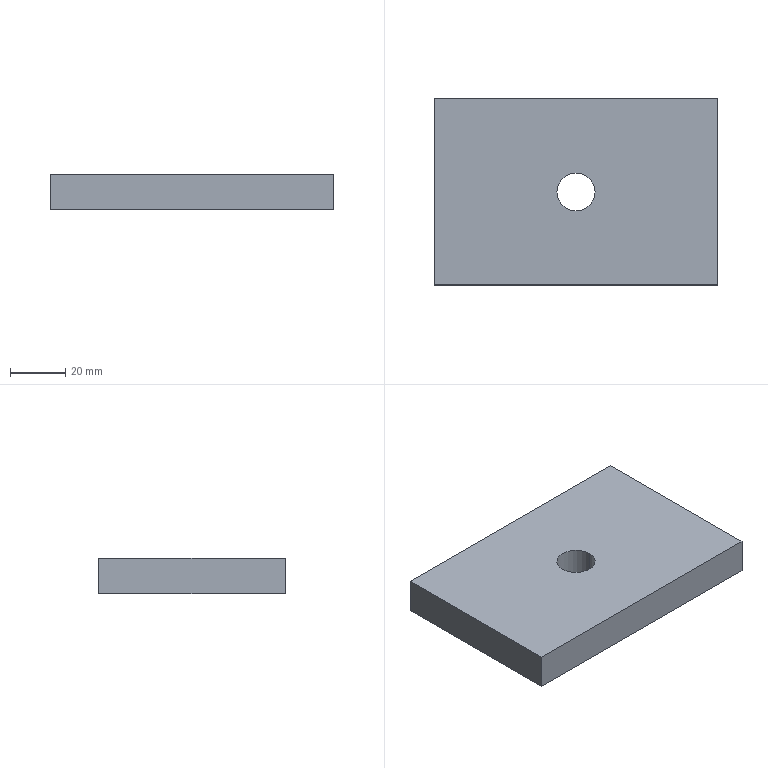Part | SolidWorks | features BaseBody 1 | 1 solid | 8 faces | box 103 x 67.6 x 13 mm | volume 88562 mm3 | plane 6 | cylinder 2 | commonest cylinder face diameters 13.835 x2
STEP:
#1=CARTESIAN_POINT('',(34.779,28.356,0.));
#2=VERTEX_POINT('',#1);
#3=CARTESIAN_POINT('',(20.944,28.356,0.));
#4=VERTEX_POINT('',#3);
#5=CARTESIAN_POINT('',(27.861,28.356,0.));
#6=DIRECTION('',(0.,0.,-1.));
#7=DIRECTION('',(1.,0.,0.));
#8=AXIS2_PLACEMENT_3D('',#5,#6,#7);
#9=CIRCLE('',#8,6.918);
#10=EDGE_CURVE('',#2,#4,#9,.T.);
#11=ORIENTED_EDGE('',*,*,#10,.T.);
#12=CARTESIAN_POINT('',(20.944,28.356,13.));
#13=VERTEX_POINT('',#12);
#14=CARTESIAN_POINT('',(20.944,28.356,-110.886));
#15=DIRECTION('',(0.,0.,1.));
#16=VECTOR('',#15,1000.);
#17=LINE('',#14,#16);
#18=EDGE_CURVE('',#4,#13,#17,.T.);
#19=ORIENTED_EDGE('',*,*,#18,.T.);
#20=CARTESIAN_POINT('',(34.779,28.356,13.));
#21=VERTEX_POINT('',#20);
#22=CARTESIAN_POINT('',(27.861,28.356,13.));
#23=DIRECTION('',(0.,0.,-1.));
#24=DIRECTION('',(1.,0.,0.));
#25=AXIS2_PLACEMENT_3D('',#22,#23,#24);
#26=CIRCLE('',#25,6.918);
#27=EDGE_CURVE('',#21,#13,#26,.T.);
#28=ORIENTED_EDGE('',*,*,#27,.F.);
#29=CARTESIAN_POINT('',(34.779,28.356,-110.886));
#30=DIRECTION('',(0.,0.,1.));
#31=VECTOR('',#30,1000.);
#32=LINE('',#29,#31);
#33=EDGE_CURVE('',#2,#21,#32,.T.);
#34=ORIENTED_EDGE('',*,*,#33,.F.);
#35=EDGE_LOOP('',(#11,#19,#28,#34));
#36=FACE_OUTER_BOUND('',#35,.T.);
#37=CARTESIAN_POINT('',(27.861,28.356,-110.886));
#38=DIRECTION('',(0.,0.,1.));
#39=DIRECTION('',(1.,0.,0.));
#40=AXIS2_PLACEMENT_3D('',#37,#38,#39);
#41=CYLINDRICAL_SURFACE('',#40,6.918);
#42=ADVANCED_FACE('',(#36),#41,.F.);
#43=ORIENTED_EDGE('',*,*,#10,.F.);
#44=CARTESIAN_POINT('',(27.861,28.356,0.));
#45=DIRECTION('',(0.,0.,-1.));
#46=DIRECTION('',(1.,0.,0.));
#47=AXIS2_PLACEMENT_3D('',#44,#45,#46);
#48=CIRCLE('',#47,6.918);
#49=EDGE_CURVE('',#4,#2,#48,.T.);
#50=ORIENTED_EDGE('',*,*,#49,.F.);
#51=EDGE_LOOP('',(#43,#50));
#52=FACE_BOUND('',#51,.T.);
#53=CARTESIAN_POINT('',(79.361,-5.444,0.));
#54=VERTEX_POINT('',#53);
#55=CARTESIAN_POINT('',(79.361,62.156,0.));
#56=VERTEX_POINT('',#55);
#57=CARTESIAN_POINT('',(79.361,28.356,0.));
#58=DIRECTION('',(0.,1.,0.));
#59=VECTOR('',#58,1000.);
#60=LINE('',#57,#59);
#61=EDGE_CURVE('',#54,#56,#60,.T.);
#62=ORIENTED_EDGE('',*,*,#61,.F.);
#63=CARTESIAN_POINT('',(-23.639,-5.444,0.));
#64=VERTEX_POINT('',#63);
#65=CARTESIAN_POINT('',(27.861,-5.444,0.));
#66=DIRECTION('',(1.,0.,0.));
#67=VECTOR('',#66,1000.);
#68=LINE('',#65,#67);
#69=EDGE_CURVE('',#64,#54,#68,.T.);
#70=ORIENTED_EDGE('',*,*,#69,.F.);
#71=CARTESIAN_POINT('',(-23.639,62.156,0.));
#72=VERTEX_POINT('',#71);
#73=CARTESIAN_POINT('',(-23.639,28.356,0.));
#74=DIRECTION('',(0.,-1.,0.));
#75=VECTOR('',#74,1000.);
#76=LINE('',#73,#75);
#77=EDGE_CURVE('',#72,#64,#76,.T.);
#78=ORIENTED_EDGE('',*,*,#77,.F.);
#79=CARTESIAN_POINT('',(27.861,62.156,0.));
#80=DIRECTION('',(-1.,0.,0.));
#81=VECTOR('',#80,1000.);
#82=LINE('',#79,#81);
#83=EDGE_CURVE('',#56,#72,#82,.T.);
#84=ORIENTED_EDGE('',*,*,#83,.F.);
#85=EDGE_LOOP('',(#62,#70,#78,#84));
#86=FACE_OUTER_BOUND('',#85,.T.);
#87=CARTESIAN_POINT('',(27.861,28.356,0.));
#88=DIRECTION('',(0.,0.,1.));
#89=DIRECTION('',(1.,0.,0.));
#90=AXIS2_PLACEMENT_3D('',#87,#88,#89);
#91=PLANE('',#90);
#92=ADVANCED_FACE('',(#52,#86),#91,.F.);
#93=ORIENTED_EDGE('',*,*,#18,.F.);
#94=ORIENTED_EDGE('',*,*,#49,.T.);
#95=ORIENTED_EDGE('',*,*,#33,.T.);
#96=CARTESIAN_POINT('',(27.861,28.356,13.));
#97=DIRECTION('',(0.,0.,-1.));
#98=DIRECTION('',(1.,0.,0.));
#99=AXIS2_PLACEMENT_3D('',#96,#97,#98);
#100=CIRCLE('',#99,6.918);
#101=EDGE_CURVE('',#13,#21,#100,.T.);
#102=ORIENTED_EDGE('',*,*,#101,.F.);
#103=EDGE_LOOP('',(#93,#94,#95,#102));
#104=FACE_OUTER_BOUND('',#103,.T.);
#105=CARTESIAN_POINT('',(27.861,28.356,-110.886));
#106=DIRECTION('',(0.,0.,1.));
#107=DIRECTION('',(1.,0.,0.));
#108=AXIS2_PLACEMENT_3D('',#105,#106,#107);
#109=CYLINDRICAL_SURFACE('',#108,6.918);
#110=ADVANCED_FACE('',(#104),#109,.F.);
#111=ORIENTED_EDGE('',*,*,#83,.T.);
#112=CARTESIAN_POINT('',(-23.639,62.156,13.));
#113=VERTEX_POINT('',#112);
#114=CARTESIAN_POINT('',(-23.639,62.156,0.));
#115=DIRECTION('',(0.,0.,1.));
#116=VECTOR('',#115,1000.);
#117=LINE('',#114,#116);
#118=EDGE_CURVE('',#72,#113,#117,.T.);
#119=ORIENTED_EDGE('',*,*,#118,.T.);
#120=CARTESIAN_POINT('',(79.361,62.156,13.));
#121=VERTEX_POINT('',#120);
#122=CARTESIAN_POINT('',(-23.639,62.156,13.));
#123=DIRECTION('',(1.,0.,0.));
#124=VECTOR('',#123,1000.);
#125=LINE('',#122,#124);
#126=EDGE_CURVE('',#113,#121,#125,.T.);
#127=ORIENTED_EDGE('',*,*,#126,.T.);
#128=CARTESIAN_POINT('',(79.361,62.156,0.));
#129=DIRECTION('',(0.,0.,-1.));
#130=VECTOR('',#129,1000.);
#131=LINE('',#128,#130);
#132=EDGE_CURVE('',#121,#56,#131,.T.);
#133=ORIENTED_EDGE('',*,*,#132,.T.);
#134=EDGE_LOOP('',(#111,#119,#127,#133));
#135=FACE_OUTER_BOUND('',#134,.T.);
#136=CARTESIAN_POINT('',(-23.639,62.156,0.));
#137=DIRECTION('',(0.,1.,0.));
#138=DIRECTION('',(0.,0.,1.));
#139=AXIS2_PLACEMENT_3D('',#136,#137,#138);
#140=PLANE('',#139);
#141=ADVANCED_FACE('',(#135),#140,.T.);
#142=ORIENTED_EDGE('',*,*,#61,.T.);
#143=ORIENTED_EDGE('',*,*,#132,.F.);
#144=CARTESIAN_POINT('',(79.361,-5.444,13.));
#145=VERTEX_POINT('',#144);
#146=CARTESIAN_POINT('',(79.361,62.156,13.));
#147=DIRECTION('',(0.,-1.,0.));
#148=VECTOR('',#147,1000.);
#149=LINE('',#146,#148);
#150=EDGE_CURVE('',#121,#145,#149,.T.);
#151=ORIENTED_EDGE('',*,*,#150,.T.);
#152=CARTESIAN_POINT('',(79.361,-5.444,0.));
#153=DIRECTION('',(0.,0.,-1.));
#154=VECTOR('',#153,1000.);
#155=LINE('',#152,#154);
#156=EDGE_CURVE('',#145,#54,#155,.T.);
#157=ORIENTED_EDGE('',*,*,#156,.T.);
#158=EDGE_LOOP('',(#142,#143,#151,#157));
#159=FACE_OUTER_BOUND('',#158,.T.);
#160=CARTESIAN_POINT('',(79.361,62.156,0.));
#161=DIRECTION('',(1.,0.,0.));
#162=DIRECTION('',(0.,0.,-1.));
#163=AXIS2_PLACEMENT_3D('',#160,#161,#162);
#164=PLANE('',#163);
#165=ADVANCED_FACE('',(#159),#164,.T.);
#166=ORIENTED_EDGE('',*,*,#69,.T.);
#167=ORIENTED_EDGE('',*,*,#156,.F.);
#168=CARTESIAN_POINT('',(-23.639,-5.444,13.));
#169=VERTEX_POINT('',#168);
#170=CARTESIAN_POINT('',(79.361,-5.444,13.));
#171=DIRECTION('',(-1.,0.,0.));
#172=VECTOR('',#171,1000.);
#173=LINE('',#170,#172);
#174=EDGE_CURVE('',#145,#169,#173,.T.);
#175=ORIENTED_EDGE('',*,*,#174,.T.);
#176=CARTESIAN_POINT('',(-23.639,-5.444,0.));
#177=DIRECTION('',(0.,0.,-1.));
#178=VECTOR('',#177,1000.);
#179=LINE('',#176,#178);
#180=EDGE_CURVE('',#169,#64,#179,.T.);
#181=ORIENTED_EDGE('',*,*,#180,.T.);
#182=EDGE_LOOP('',(#166,#167,#175,#181));
#183=FACE_OUTER_BOUND('',#182,.T.);
#184=CARTESIAN_POINT('',(79.361,-5.444,0.));
#185=DIRECTION('',(0.,-1.,0.));
#186=DIRECTION('',(1.,0.,0.));
#187=AXIS2_PLACEMENT_3D('',#184,#185,#186);
#188=PLANE('',#187);
#189=ADVANCED_FACE('',(#183),#188,.T.);
#190=ORIENTED_EDGE('',*,*,#77,.T.);
#191=ORIENTED_EDGE('',*,*,#180,.F.);
#192=CARTESIAN_POINT('',(-23.639,-5.444,13.));
#193=DIRECTION('',(0.,1.,0.));
#194=VECTOR('',#193,1000.);
#195=LINE('',#192,#194);
#196=EDGE_CURVE('',#169,#113,#195,.T.);
#197=ORIENTED_EDGE('',*,*,#196,.T.);
#198=ORIENTED_EDGE('',*,*,#118,.F.);
#199=EDGE_LOOP('',(#190,#191,#197,#198));
#200=FACE_OUTER_BOUND('',#199,.T.);
#201=CARTESIAN_POINT('',(-23.639,-5.444,0.));
#202=DIRECTION('',(-1.,0.,0.));
#203=DIRECTION('',(0.,-1.,0.));
#204=AXIS2_PLACEMENT_3D('',#201,#202,#203);
#205=PLANE('',#204);
#206=ADVANCED_FACE('',(#200),#205,.T.);
#207=ORIENTED_EDGE('',*,*,#27,.T.);
#208=ORIENTED_EDGE('',*,*,#101,.T.);
#209=EDGE_LOOP('',(#207,#208));
#210=FACE_BOUND('',#209,.T.);
#211=ORIENTED_EDGE('',*,*,#196,.F.);
#212=ORIENTED_EDGE('',*,*,#174,.F.);
#213=ORIENTED_EDGE('',*,*,#150,.F.);
#214=ORIENTED_EDGE('',*,*,#126,.F.);
#215=EDGE_LOOP('',(#211,#212,#213,#214));
#216=FACE_OUTER_BOUND('',#215,.T.);
#217=CARTESIAN_POINT('',(27.861,28.356,13.));
#218=DIRECTION('',(0.,0.,1.));
#219=DIRECTION('',(1.,0.,0.));
#220=AXIS2_PLACEMENT_3D('',#217,#218,#219);
#221=PLANE('',#220);
#222=ADVANCED_FACE('',(#210,#216),#221,.T.);
#223=CLOSED_SHELL('',(#42,#92,#110,#141,#165,#189,#206,#222));
#224=MANIFOLD_SOLID_BREP('',#223);
#225=CARTESIAN_POINT('',(0.,0.,0.));
#226=DIRECTION('',(0.,0.,1.));
#227=DIRECTION('',(1.,0.,0.));
#228=AXIS2_PLACEMENT_3D('',#225,#226,#227);
#229=(LENGTH_UNIT()NAMED_UNIT(*)SI_UNIT(.MILLI.,.METRE.));
#230=UNCERTAINTY_MEASURE_WITH_UNIT(LENGTH_MEASURE(0.00001),#229,'','');
#231=(NAMED_UNIT(*)PLANE_ANGLE_UNIT()SI_UNIT($,.RADIAN.));
#232=(NAMED_UNIT(*)SI_UNIT($,.STERADIAN.)SOLID_ANGLE_UNIT());
#233=(GEOMETRIC_REPRESENTATION_CONTEXT(3)GLOBAL_UNCERTAINTY_ASSIGNED_CONTEXT((#230))GLOBAL_UNIT_ASSIGNED_CONTEXT((#229,#231,#232))REPRESENTATION_CONTEXT('',''));
#234=ADVANCED_BREP_SHAPE_REPRESENTATION('',(#224,#228),#233);